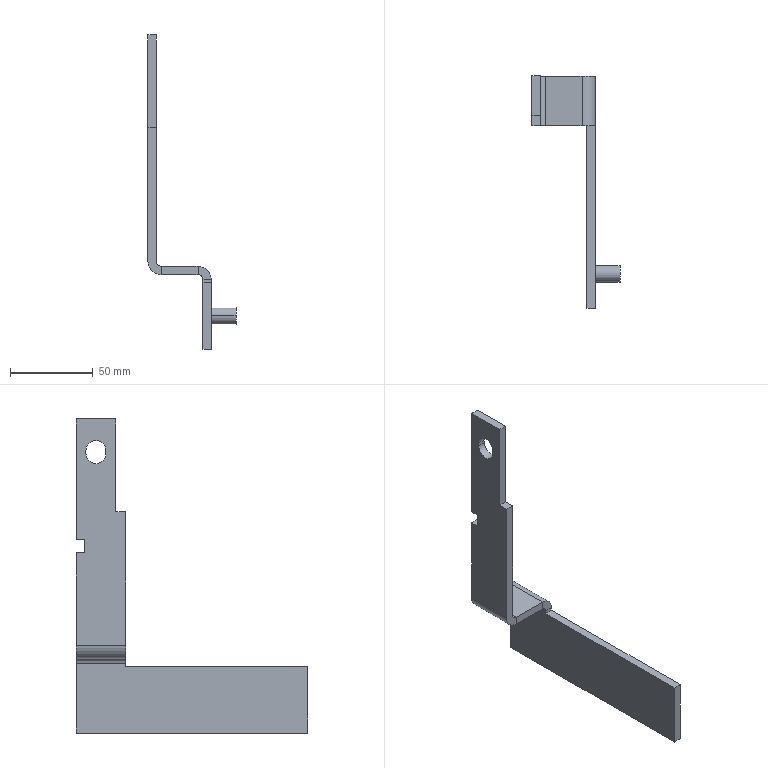Part | STEP file | 64646460 | 1 solid | 38 faces | box 53.3 x 140.3 x 190 mm | volume 53459 mm3 | plane 28 | cylinder 10 | commonest cylinder face diameters 0.1 x2 6 x2 10 x2 12 x2 16 x2